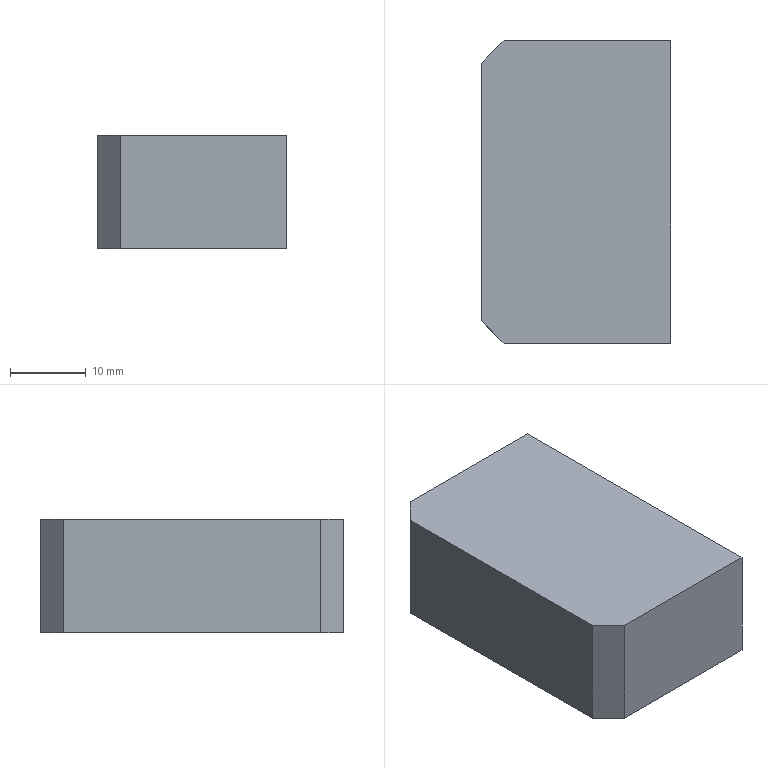Part | NX | 1 solid | 12 faces | box 25 x 40 x 15 mm | volume 14256 mm3 | plane 8 | cone 2 | cylinder 2 | commonest cylinder face diameters 5 x2
STEP:
#1=CARTESIAN_POINT('',(12.5,-15.,-2.5));
#2=VERTEX_POINT('',#1);
#3=CARTESIAN_POINT('',(12.5,-15.,0.));
#4=DIRECTION('',(1.,0.,0.));
#5=DIRECTION('',(0.,0.,-1.));
#6=AXIS2_PLACEMENT_3D('',#3,#4,#5);
#7=CIRCLE('',#6,2.5);
#8=EDGE_CURVE('',#2,#2,#7,.T.);
#9=ORIENTED_EDGE('',*,*,#8,.F.);
#10=EDGE_LOOP('',(#9));
#11=FACE_BOUND('',#10,.T.);
#12=CARTESIAN_POINT('',(12.5,15.,-2.5));
#13=VERTEX_POINT('',#12);
#14=CARTESIAN_POINT('',(12.5,15.,0.));
#15=DIRECTION('',(1.,0.,0.));
#16=DIRECTION('',(0.,0.,-1.));
#17=AXIS2_PLACEMENT_3D('',#14,#15,#16);
#18=CIRCLE('',#17,2.5);
#19=EDGE_CURVE('',#13,#13,#18,.T.);
#20=ORIENTED_EDGE('',*,*,#19,.F.);
#21=EDGE_LOOP('',(#20));
#22=FACE_BOUND('',#21,.T.);
#23=CARTESIAN_POINT('',(12.5,-20.,-7.5));
#24=VERTEX_POINT('',#23);
#25=CARTESIAN_POINT('',(12.5,20.,-7.5));
#26=VERTEX_POINT('',#25);
#27=CARTESIAN_POINT('',(12.5,20.,-7.5));
#28=DIRECTION('',(0.,1.,0.));
#29=VECTOR('',#28,1000.);
#30=LINE('',#27,#29);
#31=EDGE_CURVE('',#24,#26,#30,.T.);
#32=ORIENTED_EDGE('',*,*,#31,.T.);
#33=CARTESIAN_POINT('',(12.5,20.,7.5));
#34=VERTEX_POINT('',#33);
#35=CARTESIAN_POINT('',(12.5,20.,7.5));
#36=DIRECTION('',(0.,0.,-1.));
#37=VECTOR('',#36,1000.);
#38=LINE('',#35,#37);
#39=EDGE_CURVE('',#34,#26,#38,.T.);
#40=ORIENTED_EDGE('',*,*,#39,.F.);
#41=CARTESIAN_POINT('',(12.5,-20.,7.5));
#42=VERTEX_POINT('',#41);
#43=CARTESIAN_POINT('',(12.5,20.,7.5));
#44=DIRECTION('',(0.,1.,0.));
#45=VECTOR('',#44,1000.);
#46=LINE('',#43,#45);
#47=EDGE_CURVE('',#42,#34,#46,.T.);
#48=ORIENTED_EDGE('',*,*,#47,.F.);
#49=CARTESIAN_POINT('',(12.5,-20.,7.5));
#50=DIRECTION('',(0.,0.,-1.));
#51=VECTOR('',#50,1000.);
#52=LINE('',#49,#51);
#53=EDGE_CURVE('',#42,#24,#52,.T.);
#54=ORIENTED_EDGE('',*,*,#53,.T.);
#55=EDGE_LOOP('',(#32,#40,#48,#54));
#56=FACE_BOUND('',#55,.T.);
#57=CARTESIAN_POINT('',(12.5,20.,7.5));
#58=DIRECTION('',(-1.,0.,0.));
#59=DIRECTION('',(0.,-1.,0.));
#60=AXIS2_PLACEMENT_3D('',#57,#58,#59);
#61=PLANE('',#60);
#62=ADVANCED_FACE('',(#11,#22,#56),#61,.F.);
#63=CARTESIAN_POINT('',(-9.5,20.,-7.5));
#64=VERTEX_POINT('',#63);
#65=CARTESIAN_POINT('',(-12.5,20.,-7.5));
#66=DIRECTION('',(-1.,0.,0.));
#67=VECTOR('',#66,1000.);
#68=LINE('',#65,#67);
#69=EDGE_CURVE('',#26,#64,#68,.T.);
#70=ORIENTED_EDGE('',*,*,#69,.T.);
#71=CARTESIAN_POINT('',(-9.5,20.,7.5));
#72=VERTEX_POINT('',#71);
#73=CARTESIAN_POINT('',(-9.5,20.,7.5));
#74=DIRECTION('',(0.,0.,1.));
#75=VECTOR('',#74,1000.);
#76=LINE('',#73,#75);
#77=EDGE_CURVE('',#64,#72,#76,.T.);
#78=ORIENTED_EDGE('',*,*,#77,.T.);
#79=CARTESIAN_POINT('',(-12.5,20.,7.5));
#80=DIRECTION('',(-1.,0.,0.));
#81=VECTOR('',#80,1000.);
#82=LINE('',#79,#81);
#83=EDGE_CURVE('',#34,#72,#82,.T.);
#84=ORIENTED_EDGE('',*,*,#83,.F.);
#85=ORIENTED_EDGE('',*,*,#39,.T.);
#86=EDGE_LOOP('',(#70,#78,#84,#85));
#87=FACE_BOUND('',#86,.T.);
#88=CARTESIAN_POINT('',(-12.5,20.,7.5));
#89=DIRECTION('',(0.,-1.,0.));
#90=DIRECTION('',(0.,0.,-1.));
#91=AXIS2_PLACEMENT_3D('',#88,#89,#90);
#92=PLANE('',#91);
#93=ADVANCED_FACE('',(#87),#92,.F.);
#94=CARTESIAN_POINT('',(-12.5,17.,7.5));
#95=VERTEX_POINT('',#94);
#96=CARTESIAN_POINT('',(-12.5,-17.,7.5));
#97=VERTEX_POINT('',#96);
#98=CARTESIAN_POINT('',(-12.5,20.,7.5));
#99=DIRECTION('',(0.,-1.,0.));
#100=VECTOR('',#99,1000.);
#101=LINE('',#98,#100);
#102=EDGE_CURVE('',#95,#97,#101,.T.);
#103=ORIENTED_EDGE('',*,*,#102,.F.);
#104=CARTESIAN_POINT('',(-12.5,17.,-7.5));
#105=VERTEX_POINT('',#104);
#106=CARTESIAN_POINT('',(-12.5,17.,7.5));
#107=DIRECTION('',(0.,0.,-1.));
#108=VECTOR('',#107,1000.);
#109=LINE('',#106,#108);
#110=EDGE_CURVE('',#95,#105,#109,.T.);
#111=ORIENTED_EDGE('',*,*,#110,.T.);
#112=CARTESIAN_POINT('',(-12.5,-17.,-7.5));
#113=VERTEX_POINT('',#112);
#114=CARTESIAN_POINT('',(-12.5,20.,-7.5));
#115=DIRECTION('',(0.,-1.,0.));
#116=VECTOR('',#115,1000.);
#117=LINE('',#114,#116);
#118=EDGE_CURVE('',#105,#113,#117,.T.);
#119=ORIENTED_EDGE('',*,*,#118,.T.);
#120=CARTESIAN_POINT('',(-12.5,-17.,7.5));
#121=DIRECTION('',(0.,0.,1.));
#122=VECTOR('',#121,1000.);
#123=LINE('',#120,#122);
#124=EDGE_CURVE('',#113,#97,#123,.T.);
#125=ORIENTED_EDGE('',*,*,#124,.T.);
#126=EDGE_LOOP('',(#103,#111,#119,#125));
#127=FACE_BOUND('',#126,.T.);
#128=CARTESIAN_POINT('',(-12.5,20.,7.5));
#129=DIRECTION('',(1.,0.,0.));
#130=DIRECTION('',(0.,1.,0.));
#131=AXIS2_PLACEMENT_3D('',#128,#129,#130);
#132=PLANE('',#131);
#133=ADVANCED_FACE('',(#127),#132,.F.);
#134=CARTESIAN_POINT('',(-9.5,-20.,7.5));
#135=VERTEX_POINT('',#134);
#136=CARTESIAN_POINT('',(-12.5,-20.,7.5));
#137=DIRECTION('',(1.,0.,0.));
#138=VECTOR('',#137,1000.);
#139=LINE('',#136,#138);
#140=EDGE_CURVE('',#135,#42,#139,.T.);
#141=ORIENTED_EDGE('',*,*,#140,.F.);
#142=CARTESIAN_POINT('',(-9.5,-20.,-7.5));
#143=VERTEX_POINT('',#142);
#144=CARTESIAN_POINT('',(-9.5,-20.,7.5));
#145=DIRECTION('',(0.,0.,-1.));
#146=VECTOR('',#145,1000.);
#147=LINE('',#144,#146);
#148=EDGE_CURVE('',#135,#143,#147,.T.);
#149=ORIENTED_EDGE('',*,*,#148,.T.);
#150=CARTESIAN_POINT('',(-12.5,-20.,-7.5));
#151=DIRECTION('',(1.,0.,0.));
#152=VECTOR('',#151,1000.);
#153=LINE('',#150,#152);
#154=EDGE_CURVE('',#143,#24,#153,.T.);
#155=ORIENTED_EDGE('',*,*,#154,.T.);
#156=ORIENTED_EDGE('',*,*,#53,.F.);
#157=EDGE_LOOP('',(#141,#149,#155,#156));
#158=FACE_BOUND('',#157,.T.);
#159=CARTESIAN_POINT('',(-12.5,-20.,7.5));
#160=DIRECTION('',(0.,1.,0.));
#161=DIRECTION('',(0.,0.,1.));
#162=AXIS2_PLACEMENT_3D('',#159,#160,#161);
#163=PLANE('',#162);
#164=ADVANCED_FACE('',(#158),#163,.F.);
#165=ORIENTED_EDGE('',*,*,#83,.T.);
#166=CARTESIAN_POINT('',(-14.75,14.75,7.5));
#167=DIRECTION('',(0.7071,0.7071,0.));
#168=VECTOR('',#167,1000.);
#169=LINE('',#166,#168);
#170=EDGE_CURVE('',#72,#95,#169,.F.);
#171=ORIENTED_EDGE('',*,*,#170,.T.);
#172=ORIENTED_EDGE('',*,*,#102,.T.);
#173=CARTESIAN_POINT('',(-14.75,-14.75,7.5));
#174=DIRECTION('',(-0.7071,0.7071,0.));
#175=VECTOR('',#174,1000.);
#176=LINE('',#173,#175);
#177=EDGE_CURVE('',#97,#135,#176,.F.);
#178=ORIENTED_EDGE('',*,*,#177,.T.);
#179=ORIENTED_EDGE('',*,*,#140,.T.);
#180=ORIENTED_EDGE('',*,*,#47,.T.);
#181=EDGE_LOOP('',(#165,#171,#172,#178,#179,#180));
#182=FACE_BOUND('',#181,.T.);
#183=CARTESIAN_POINT('',(0.,0.,7.5));
#184=DIRECTION('',(0.,0.,1.));
#185=DIRECTION('',(1.,0.,0.));
#186=AXIS2_PLACEMENT_3D('',#183,#184,#185);
#187=PLANE('',#186);
#188=ADVANCED_FACE('',(#182),#187,.T.);
#189=ORIENTED_EDGE('',*,*,#118,.F.);
#190=CARTESIAN_POINT('',(-12.5,17.,-7.5));
#191=DIRECTION('',(-0.7071,-0.7071,0.));
#192=VECTOR('',#191,1000.);
#193=LINE('',#190,#192);
#194=EDGE_CURVE('',#105,#64,#193,.F.);
#195=ORIENTED_EDGE('',*,*,#194,.T.);
#196=ORIENTED_EDGE('',*,*,#69,.F.);
#197=ORIENTED_EDGE('',*,*,#31,.F.);
#198=ORIENTED_EDGE('',*,*,#154,.F.);
#199=CARTESIAN_POINT('',(-9.5,-20.,-7.5));
#200=DIRECTION('',(0.7071,-0.7071,0.));
#201=VECTOR('',#200,1000.);
#202=LINE('',#199,#201);
#203=EDGE_CURVE('',#143,#113,#202,.F.);
#204=ORIENTED_EDGE('',*,*,#203,.T.);
#205=EDGE_LOOP('',(#189,#195,#196,#197,#198,#204));
#206=FACE_BOUND('',#205,.T.);
#207=CARTESIAN_POINT('',(0.,0.,-7.5));
#208=DIRECTION('',(0.,0.,1.));
#209=DIRECTION('',(1.,0.,0.));
#210=AXIS2_PLACEMENT_3D('',#207,#208,#209);
#211=PLANE('',#210);
#212=ADVANCED_FACE('',(#206),#211,.F.);
#213=CARTESIAN_POINT('',(-4.002,15.,0.));
#214=VERTEX_POINT('',#213);
#215=VERTEX_LOOP('',#214);
#216=FACE_BOUND('',#215,.T.);
#217=CARTESIAN_POINT('',(-2.5,15.,-2.5));
#218=VERTEX_POINT('',#217);
#219=CARTESIAN_POINT('',(-2.5,15.,0.));
#220=DIRECTION('',(1.,0.,0.));
#221=DIRECTION('',(0.,0.,-1.));
#222=AXIS2_PLACEMENT_3D('',#219,#220,#221);
#223=CIRCLE('',#222,2.5);
#224=EDGE_CURVE('',#218,#218,#223,.T.);
#225=ORIENTED_EDGE('',*,*,#224,.T.);
#226=EDGE_LOOP('',(#225));
#227=FACE_BOUND('',#226,.T.);
#228=CARTESIAN_POINT('',(-2.5,15.,0.));
#229=DIRECTION('',(1.,0.,0.));
#230=DIRECTION('',(0.,0.,-1.));
#231=AXIS2_PLACEMENT_3D('',#228,#229,#230);
#232=CONICAL_SURFACE('',#231,2.5,1.03);
#233=ADVANCED_FACE('',(#216,#227),#232,.F.);
#234=ORIENTED_EDGE('',*,*,#224,.F.);
#235=EDGE_LOOP('',(#234));
#236=FACE_BOUND('',#235,.T.);
#237=ORIENTED_EDGE('',*,*,#19,.T.);
#238=EDGE_LOOP('',(#237));
#239=FACE_BOUND('',#238,.T.);
#240=CARTESIAN_POINT('',(12.5,15.,0.));
#241=DIRECTION('',(1.,0.,0.));
#242=DIRECTION('',(0.,0.,-1.));
#243=AXIS2_PLACEMENT_3D('',#240,#241,#242);
#244=CYLINDRICAL_SURFACE('',#243,2.5);
#245=ADVANCED_FACE('',(#236,#239),#244,.F.);
#246=CARTESIAN_POINT('',(-4.002,-15.,0.));
#247=VERTEX_POINT('',#246);
#248=VERTEX_LOOP('',#247);
#249=FACE_BOUND('',#248,.T.);
#250=CARTESIAN_POINT('',(-2.5,-15.,-2.5));
#251=VERTEX_POINT('',#250);
#252=CARTESIAN_POINT('',(-2.5,-15.,0.));
#253=DIRECTION('',(1.,0.,0.));
#254=DIRECTION('',(0.,0.,-1.));
#255=AXIS2_PLACEMENT_3D('',#252,#253,#254);
#256=CIRCLE('',#255,2.5);
#257=EDGE_CURVE('',#251,#251,#256,.T.);
#258=ORIENTED_EDGE('',*,*,#257,.T.);
#259=EDGE_LOOP('',(#258));
#260=FACE_BOUND('',#259,.T.);
#261=CARTESIAN_POINT('',(-2.5,-15.,0.));
#262=DIRECTION('',(1.,0.,0.));
#263=DIRECTION('',(0.,0.,-1.));
#264=AXIS2_PLACEMENT_3D('',#261,#262,#263);
#265=CONICAL_SURFACE('',#264,2.5,1.03);
#266=ADVANCED_FACE('',(#249,#260),#265,.F.);
#267=ORIENTED_EDGE('',*,*,#257,.F.);
#268=EDGE_LOOP('',(#267));
#269=FACE_BOUND('',#268,.T.);
#270=ORIENTED_EDGE('',*,*,#8,.T.);
#271=EDGE_LOOP('',(#270));
#272=FACE_BOUND('',#271,.T.);
#273=CARTESIAN_POINT('',(12.5,-15.,0.));
#274=DIRECTION('',(1.,0.,0.));
#275=DIRECTION('',(0.,0.,-1.));
#276=AXIS2_PLACEMENT_3D('',#273,#274,#275);
#277=CYLINDRICAL_SURFACE('',#276,2.5);
#278=ADVANCED_FACE('',(#269,#272),#277,.F.);
#279=ORIENTED_EDGE('',*,*,#170,.F.);
#280=ORIENTED_EDGE('',*,*,#77,.F.);
#281=ORIENTED_EDGE('',*,*,#194,.F.);
#282=ORIENTED_EDGE('',*,*,#110,.F.);
#283=EDGE_LOOP('',(#279,#280,#281,#282));
#284=FACE_BOUND('',#283,.T.);
#285=CARTESIAN_POINT('',(-12.5,17.,7.5));
#286=DIRECTION('',(0.7071,-0.7071,0.));
#287=DIRECTION('',(0.,0.,-1.));
#288=AXIS2_PLACEMENT_3D('',#285,#286,#287);
#289=PLANE('',#288);
#290=ADVANCED_FACE('',(#284),#289,.F.);
#291=ORIENTED_EDGE('',*,*,#177,.F.);
#292=ORIENTED_EDGE('',*,*,#124,.F.);
#293=ORIENTED_EDGE('',*,*,#203,.F.);
#294=ORIENTED_EDGE('',*,*,#148,.F.);
#295=EDGE_LOOP('',(#291,#292,#293,#294));
#296=FACE_BOUND('',#295,.T.);
#297=CARTESIAN_POINT('',(-9.5,-20.,7.5));
#298=DIRECTION('',(0.7071,0.7071,0.));
#299=DIRECTION('',(0.,0.,-1.));
#300=AXIS2_PLACEMENT_3D('',#297,#298,#299);
#301=PLANE('',#300);
#302=ADVANCED_FACE('',(#296),#301,.F.);
#303=CLOSED_SHELL('',(#62,#93,#133,#164,#188,#212,#233,#245,#266,#278,#290,#302));
#304=MANIFOLD_SOLID_BREP('',#303);
#305=(LENGTH_UNIT()NAMED_UNIT(*)SI_UNIT(.MILLI.,.METRE.));
#306=UNCERTAINTY_MEASURE_WITH_UNIT(LENGTH_MEASURE(0.00001),#305,'','');
#307=(NAMED_UNIT(*)PLANE_ANGLE_UNIT()SI_UNIT($,.RADIAN.));
#308=(NAMED_UNIT(*)SI_UNIT($,.STERADIAN.)SOLID_ANGLE_UNIT());
#309=(GEOMETRIC_REPRESENTATION_CONTEXT(3)GLOBAL_UNCERTAINTY_ASSIGNED_CONTEXT((#306))GLOBAL_UNIT_ASSIGNED_CONTEXT((#305,#307,#308))REPRESENTATION_CONTEXT('',''));
#310=ADVANCED_BREP_SHAPE_REPRESENTATION('',(#304),#309);